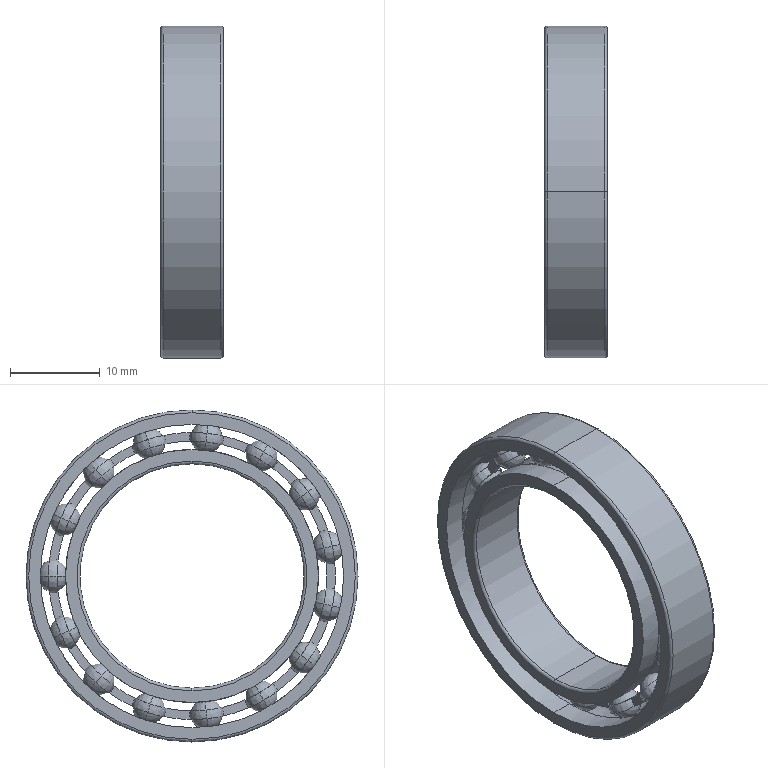Part | SolidWorks | features Revolution 5, CirPattern 2, RevCut 2 | 1 solid | 226 faces | box 7 x 37 x 37 mm | volume 2477 mm3 | sphere 120 | torus 56 | plane 34 | cylinder 16 | commonest cylinder face diameters 28.2 x4 33.8 x4 25 x2 30.038 x2 31.963 x2 37 x2